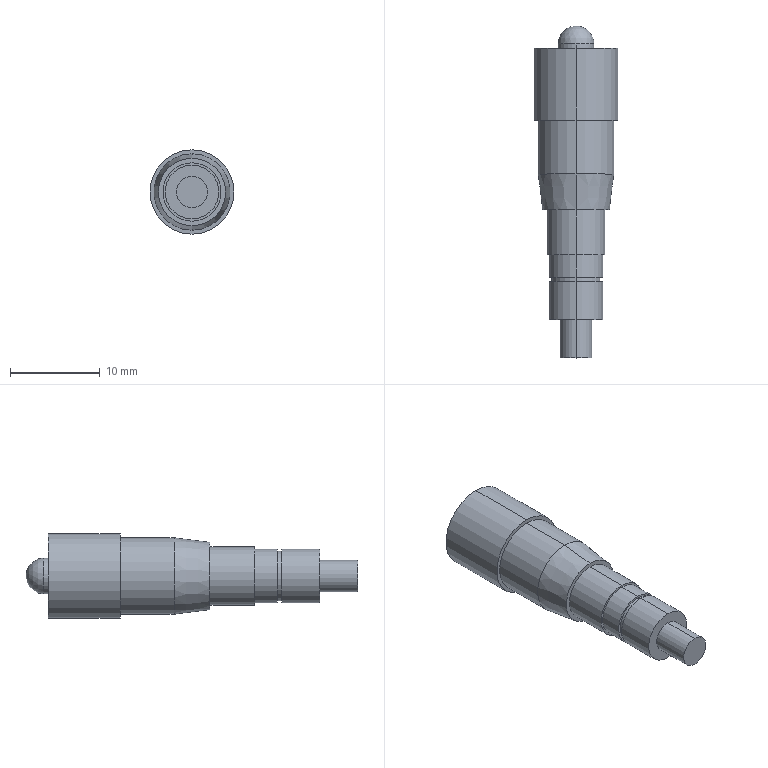Part | SolidWorks | features ICE 7, Chamfer 1, Extrusion 1, Fillet 1 | 1 solid | 27 faces | box 9.4 x 37 x 9.4 mm | volume 1530 mm3 | cylinder 16 | plane 8 | cone 2 | sphere 1 | commonest cylinder face diameters 6 x4 3.5 x2 4 x2 5.5 x2 6.5 x2 8.5 x2
STEP:
#1=CARTESIAN_POINT('',(0.,35.,-2.));
#2=VERTEX_POINT('',#1);
#3=CARTESIAN_POINT('',(0.,35.,2.));
#4=VERTEX_POINT('',#3);
#5=CARTESIAN_POINT('',(0.,35.,0.));
#6=DIRECTION('',(0.,-1.,0.));
#7=DIRECTION('',(0.,0.,-1.));
#8=AXIS2_PLACEMENT_3D('',#5,#6,#7);
#9=CIRCLE('',#8,2.);
#10=EDGE_CURVE('',#2,#4,#9,.T.);
#11=ORIENTED_EDGE('',*,*,#10,.T.);
#12=CARTESIAN_POINT('',(0.,34.5,2.));
#13=VERTEX_POINT('',#12);
#14=CARTESIAN_POINT('',(0.,37.,2.));
#15=DIRECTION('',(0.,-1.,0.));
#16=VECTOR('',#15,1000.);
#17=LINE('',#14,#16);
#18=EDGE_CURVE('',#4,#13,#17,.T.);
#19=ORIENTED_EDGE('',*,*,#18,.T.);
#20=CARTESIAN_POINT('',(0.,34.5,-2.));
#21=VERTEX_POINT('',#20);
#22=CARTESIAN_POINT('',(0.,34.5,0.));
#23=DIRECTION('',(0.,1.,0.));
#24=DIRECTION('',(0.,0.,1.));
#25=AXIS2_PLACEMENT_3D('',#22,#23,#24);
#26=CIRCLE('',#25,2.);
#27=EDGE_CURVE('',#13,#21,#26,.T.);
#28=ORIENTED_EDGE('',*,*,#27,.T.);
#29=CARTESIAN_POINT('',(0.,37.,-2.));
#30=DIRECTION('',(0.,-1.,0.));
#31=VECTOR('',#30,1000.);
#32=LINE('',#29,#31);
#33=EDGE_CURVE('',#2,#21,#32,.T.);
#34=ORIENTED_EDGE('',*,*,#33,.F.);
#35=EDGE_LOOP('',(#11,#19,#28,#34));
#36=FACE_OUTER_BOUND('',#35,.T.);
#37=CARTESIAN_POINT('',(0.,37.,0.));
#38=DIRECTION('',(0.,-1.,0.));
#39=DIRECTION('',(0.,0.,-1.));
#40=AXIS2_PLACEMENT_3D('',#37,#38,#39);
#41=CYLINDRICAL_SURFACE('',#40,2.);
#42=ADVANCED_FACE('',(#36),#41,.T.);
#43=CARTESIAN_POINT('',(0.,34.5,4.7));
#44=VERTEX_POINT('',#43);
#45=CARTESIAN_POINT('',(0.,34.5,-4.7));
#46=VERTEX_POINT('',#45);
#47=CARTESIAN_POINT('',(0.,34.5,0.));
#48=DIRECTION('',(0.,1.,0.));
#49=DIRECTION('',(0.,0.,1.));
#50=AXIS2_PLACEMENT_3D('',#47,#48,#49);
#51=CIRCLE('',#50,4.7);
#52=EDGE_CURVE('',#44,#46,#51,.T.);
#53=ORIENTED_EDGE('',*,*,#52,.F.);
#54=CARTESIAN_POINT('',(0.,26.5,4.7));
#55=VERTEX_POINT('',#54);
#56=CARTESIAN_POINT('',(0.,34.5,4.7));
#57=DIRECTION('',(0.,-1.,0.));
#58=VECTOR('',#57,1000.);
#59=LINE('',#56,#58);
#60=EDGE_CURVE('',#44,#55,#59,.T.);
#61=ORIENTED_EDGE('',*,*,#60,.T.);
#62=CARTESIAN_POINT('',(0.,26.5,-4.7));
#63=VERTEX_POINT('',#62);
#64=CARTESIAN_POINT('',(0.,26.5,0.));
#65=DIRECTION('',(0.,1.,0.));
#66=DIRECTION('',(0.,0.,1.));
#67=AXIS2_PLACEMENT_3D('',#64,#65,#66);
#68=CIRCLE('',#67,4.7);
#69=EDGE_CURVE('',#55,#63,#68,.T.);
#70=ORIENTED_EDGE('',*,*,#69,.T.);
#71=CARTESIAN_POINT('',(0.,34.5,-4.7));
#72=DIRECTION('',(0.,-1.,0.));
#73=VECTOR('',#72,1000.);
#74=LINE('',#71,#73);
#75=EDGE_CURVE('',#46,#63,#74,.T.);
#76=ORIENTED_EDGE('',*,*,#75,.F.);
#77=EDGE_LOOP('',(#53,#61,#70,#76));
#78=FACE_OUTER_BOUND('',#77,.T.);
#79=CARTESIAN_POINT('',(0.,34.5,0.));
#80=DIRECTION('',(0.,-1.,0.));
#81=DIRECTION('',(0.,0.,-1.));
#82=AXIS2_PLACEMENT_3D('',#79,#80,#81);
#83=CYLINDRICAL_SURFACE('',#82,4.7);
#84=ADVANCED_FACE('',(#78),#83,.T.);
#85=CARTESIAN_POINT('',(0.,16.5,-3.75));
#86=VERTEX_POINT('',#85);
#87=CARTESIAN_POINT('',(0.,16.5,3.75));
#88=VERTEX_POINT('',#87);
#89=CARTESIAN_POINT('',(0.,16.5,0.));
#90=DIRECTION('',(0.,-1.,0.));
#91=DIRECTION('',(0.,0.,1.));
#92=AXIS2_PLACEMENT_3D('',#89,#90,#91);
#93=CIRCLE('',#92,3.75);
#94=EDGE_CURVE('',#86,#88,#93,.T.);
#95=ORIENTED_EDGE('',*,*,#94,.F.);
#96=CARTESIAN_POINT('',(0.,20.5,-4.25));
#97=VERTEX_POINT('',#96);
#98=CARTESIAN_POINT('',(0.,20.5,-4.25));
#99=DIRECTION('',(0.,0.9923,-0.124));
#100=VECTOR('',#99,1000.);
#101=LINE('',#98,#100);
#102=EDGE_CURVE('',#86,#97,#101,.T.);
#103=ORIENTED_EDGE('',*,*,#102,.T.);
#104=CARTESIAN_POINT('',(0.,20.5,4.25));
#105=VERTEX_POINT('',#104);
#106=CARTESIAN_POINT('',(0.,20.5,0.));
#107=DIRECTION('',(0.,1.,0.));
#108=DIRECTION('',(0.,0.,1.));
#109=AXIS2_PLACEMENT_3D('',#106,#107,#108);
#110=CIRCLE('',#109,4.25);
#111=EDGE_CURVE('',#105,#97,#110,.T.);
#112=ORIENTED_EDGE('',*,*,#111,.F.);
#113=CARTESIAN_POINT('',(0.,20.5,4.25));
#114=DIRECTION('',(0.,0.9923,0.124));
#115=VECTOR('',#114,1000.);
#116=LINE('',#113,#115);
#117=EDGE_CURVE('',#88,#105,#116,.T.);
#118=ORIENTED_EDGE('',*,*,#117,.F.);
#119=EDGE_LOOP('',(#95,#103,#112,#118));
#120=FACE_OUTER_BOUND('',#119,.T.);
#121=CARTESIAN_POINT('',(0.,20.5,0.));
#122=DIRECTION('',(0.,1.,0.));
#123=DIRECTION('',(0.,0.,1.));
#124=AXIS2_PLACEMENT_3D('',#121,#122,#123);
#125=CONICAL_SURFACE('',#124,4.25,0.1244);
#126=ADVANCED_FACE('',(#120),#125,.T.);
#127=CARTESIAN_POINT('',(0.,26.5,4.25));
#128=VERTEX_POINT('',#127);
#129=CARTESIAN_POINT('',(0.,26.5,-4.25));
#130=VERTEX_POINT('',#129);
#131=CARTESIAN_POINT('',(0.,26.5,0.));
#132=DIRECTION('',(0.,1.,0.));
#133=DIRECTION('',(0.,0.,1.));
#134=AXIS2_PLACEMENT_3D('',#131,#132,#133);
#135=CIRCLE('',#134,4.25);
#136=EDGE_CURVE('',#128,#130,#135,.T.);
#137=ORIENTED_EDGE('',*,*,#136,.F.);
#138=CARTESIAN_POINT('',(0.,26.5,4.25));
#139=DIRECTION('',(0.,-1.,0.));
#140=VECTOR('',#139,1000.);
#141=LINE('',#138,#140);
#142=EDGE_CURVE('',#128,#105,#141,.T.);
#143=ORIENTED_EDGE('',*,*,#142,.T.);
#144=ORIENTED_EDGE('',*,*,#111,.T.);
#145=CARTESIAN_POINT('',(0.,26.5,-4.25));
#146=DIRECTION('',(0.,-1.,0.));
#147=VECTOR('',#146,1000.);
#148=LINE('',#145,#147);
#149=EDGE_CURVE('',#130,#97,#148,.T.);
#150=ORIENTED_EDGE('',*,*,#149,.F.);
#151=EDGE_LOOP('',(#137,#143,#144,#150));
#152=FACE_OUTER_BOUND('',#151,.T.);
#153=CARTESIAN_POINT('',(0.,26.5,0.));
#154=DIRECTION('',(0.,-1.,0.));
#155=DIRECTION('',(0.,0.,-1.));
#156=AXIS2_PLACEMENT_3D('',#153,#154,#155);
#157=CYLINDRICAL_SURFACE('',#156,4.25);
#158=ADVANCED_FACE('',(#152),#157,.T.);
#159=CARTESIAN_POINT('',(0.,16.5,3.25));
#160=VERTEX_POINT('',#159);
#161=CARTESIAN_POINT('',(0.,16.5,-3.25));
#162=VERTEX_POINT('',#161);
#163=CARTESIAN_POINT('',(0.,16.5,0.));
#164=DIRECTION('',(0.,1.,0.));
#165=DIRECTION('',(0.,0.,1.));
#166=AXIS2_PLACEMENT_3D('',#163,#164,#165);
#167=CIRCLE('',#166,3.25);
#168=EDGE_CURVE('',#160,#162,#167,.T.);
#169=ORIENTED_EDGE('',*,*,#168,.F.);
#170=CARTESIAN_POINT('',(0.,11.5,3.25));
#171=VERTEX_POINT('',#170);
#172=CARTESIAN_POINT('',(0.,16.5,3.25));
#173=DIRECTION('',(0.,-1.,0.));
#174=VECTOR('',#173,1000.);
#175=LINE('',#172,#174);
#176=EDGE_CURVE('',#160,#171,#175,.T.);
#177=ORIENTED_EDGE('',*,*,#176,.T.);
#178=CARTESIAN_POINT('',(0.,11.5,-3.25));
#179=VERTEX_POINT('',#178);
#180=CARTESIAN_POINT('',(0.,11.5,0.));
#181=DIRECTION('',(0.,1.,0.));
#182=DIRECTION('',(0.,0.,1.));
#183=AXIS2_PLACEMENT_3D('',#180,#181,#182);
#184=CIRCLE('',#183,3.25);
#185=EDGE_CURVE('',#171,#179,#184,.T.);
#186=ORIENTED_EDGE('',*,*,#185,.T.);
#187=CARTESIAN_POINT('',(0.,16.5,-3.25));
#188=DIRECTION('',(0.,-1.,0.));
#189=VECTOR('',#188,1000.);
#190=LINE('',#187,#189);
#191=EDGE_CURVE('',#162,#179,#190,.T.);
#192=ORIENTED_EDGE('',*,*,#191,.F.);
#193=EDGE_LOOP('',(#169,#177,#186,#192));
#194=FACE_OUTER_BOUND('',#193,.T.);
#195=CARTESIAN_POINT('',(0.,16.5,0.));
#196=DIRECTION('',(0.,-1.,0.));
#197=DIRECTION('',(0.,0.,-1.));
#198=AXIS2_PLACEMENT_3D('',#195,#196,#197);
#199=CYLINDRICAL_SURFACE('',#198,3.25);
#200=ADVANCED_FACE('',(#194),#199,.T.);
#201=CARTESIAN_POINT('',(0.,11.5,3.));
#202=VERTEX_POINT('',#201);
#203=CARTESIAN_POINT('',(0.,11.5,-3.));
#204=VERTEX_POINT('',#203);
#205=CARTESIAN_POINT('',(0.,11.5,0.));
#206=DIRECTION('',(0.,1.,0.));
#207=DIRECTION('',(0.,0.,1.));
#208=AXIS2_PLACEMENT_3D('',#205,#206,#207);
#209=CIRCLE('',#208,3.);
#210=EDGE_CURVE('',#202,#204,#209,.T.);
#211=ORIENTED_EDGE('',*,*,#210,.F.);
#212=CARTESIAN_POINT('',(0.,9.,3.));
#213=VERTEX_POINT('',#212);
#214=CARTESIAN_POINT('',(0.,11.5,3.));
#215=DIRECTION('',(0.,-1.,0.));
#216=VECTOR('',#215,1000.);
#217=LINE('',#214,#216);
#218=EDGE_CURVE('',#202,#213,#217,.T.);
#219=ORIENTED_EDGE('',*,*,#218,.T.);
#220=CARTESIAN_POINT('',(0.,9.,-3.));
#221=VERTEX_POINT('',#220);
#222=CARTESIAN_POINT('',(0.,9.,0.));
#223=DIRECTION('',(0.,1.,0.));
#224=DIRECTION('',(0.,0.,1.));
#225=AXIS2_PLACEMENT_3D('',#222,#223,#224);
#226=CIRCLE('',#225,3.);
#227=EDGE_CURVE('',#213,#221,#226,.T.);
#228=ORIENTED_EDGE('',*,*,#227,.T.);
#229=CARTESIAN_POINT('',(0.,11.5,-3.));
#230=DIRECTION('',(0.,-1.,0.));
#231=VECTOR('',#230,1000.);
#232=LINE('',#229,#231);
#233=EDGE_CURVE('',#204,#221,#232,.T.);
#234=ORIENTED_EDGE('',*,*,#233,.F.);
#235=EDGE_LOOP('',(#211,#219,#228,#234));
#236=FACE_OUTER_BOUND('',#235,.T.);
#237=CARTESIAN_POINT('',(0.,11.5,0.));
#238=DIRECTION('',(0.,-1.,0.));
#239=DIRECTION('',(0.,0.,-1.));
#240=AXIS2_PLACEMENT_3D('',#237,#238,#239);
#241=CYLINDRICAL_SURFACE('',#240,3.);
#242=ADVANCED_FACE('',(#236),#241,.T.);
#243=CARTESIAN_POINT('',(0.,9.,2.75));
#244=VERTEX_POINT('',#243);
#245=CARTESIAN_POINT('',(0.,9.,-2.75));
#246=VERTEX_POINT('',#245);
#247=CARTESIAN_POINT('',(0.,9.,0.));
#248=DIRECTION('',(0.,1.,0.));
#249=DIRECTION('',(0.,0.,1.));
#250=AXIS2_PLACEMENT_3D('',#247,#248,#249);
#251=CIRCLE('',#250,2.75);
#252=EDGE_CURVE('',#244,#246,#251,.T.);
#253=ORIENTED_EDGE('',*,*,#252,.F.);
#254=CARTESIAN_POINT('',(0.,8.5,2.75));
#255=VERTEX_POINT('',#254);
#256=CARTESIAN_POINT('',(0.,9.,2.75));
#257=DIRECTION('',(0.,-1.,0.));
#258=VECTOR('',#257,1000.);
#259=LINE('',#256,#258);
#260=EDGE_CURVE('',#244,#255,#259,.T.);
#261=ORIENTED_EDGE('',*,*,#260,.T.);
#262=CARTESIAN_POINT('',(0.,8.5,-2.75));
#263=VERTEX_POINT('',#262);
#264=CARTESIAN_POINT('',(0.,8.5,0.));
#265=DIRECTION('',(0.,1.,0.));
#266=DIRECTION('',(0.,0.,1.));
#267=AXIS2_PLACEMENT_3D('',#264,#265,#266);
#268=CIRCLE('',#267,2.75);
#269=EDGE_CURVE('',#255,#263,#268,.T.);
#270=ORIENTED_EDGE('',*,*,#269,.T.);
#271=CARTESIAN_POINT('',(0.,9.,-2.75));
#272=DIRECTION('',(0.,-1.,0.));
#273=VECTOR('',#272,1000.);
#274=LINE('',#271,#273);
#275=EDGE_CURVE('',#246,#263,#274,.T.);
#276=ORIENTED_EDGE('',*,*,#275,.F.);
#277=EDGE_LOOP('',(#253,#261,#270,#276));
#278=FACE_OUTER_BOUND('',#277,.T.);
#279=CARTESIAN_POINT('',(0.,9.,0.));
#280=DIRECTION('',(0.,-1.,0.));
#281=DIRECTION('',(0.,0.,-1.));
#282=AXIS2_PLACEMENT_3D('',#279,#280,#281);
#283=CYLINDRICAL_SURFACE('',#282,2.75);
#284=ADVANCED_FACE('',(#278),#283,.T.);
#285=CARTESIAN_POINT('',(0.,8.5,3.));
#286=VERTEX_POINT('',#285);
#287=CARTESIAN_POINT('',(0.,8.5,-3.));
#288=VERTEX_POINT('',#287);
#289=CARTESIAN_POINT('',(0.,8.5,0.));
#290=DIRECTION('',(0.,1.,0.));
#291=DIRECTION('',(0.,0.,1.));
#292=AXIS2_PLACEMENT_3D('',#289,#290,#291);
#293=CIRCLE('',#292,3.);
#294=EDGE_CURVE('',#286,#288,#293,.T.);
#295=ORIENTED_EDGE('',*,*,#294,.F.);
#296=CARTESIAN_POINT('',(0.,4.25,3.));
#297=VERTEX_POINT('',#296);
#298=CARTESIAN_POINT('',(0.,8.5,3.));
#299=DIRECTION('',(0.,-1.,0.));
#300=VECTOR('',#299,1000.);
#301=LINE('',#298,#300);
#302=EDGE_CURVE('',#286,#297,#301,.T.);
#303=ORIENTED_EDGE('',*,*,#302,.T.);
#304=CARTESIAN_POINT('',(0.,4.25,-3.));
#305=VERTEX_POINT('',#304);
#306=CARTESIAN_POINT('',(0.,4.25,0.));
#307=DIRECTION('',(0.,1.,0.));
#308=DIRECTION('',(0.,0.,1.));
#309=AXIS2_PLACEMENT_3D('',#306,#307,#308);
#310=CIRCLE('',#309,3.);
#311=EDGE_CURVE('',#297,#305,#310,.T.);
#312=ORIENTED_EDGE('',*,*,#311,.T.);
#313=CARTESIAN_POINT('',(0.,8.5,-3.));
#314=DIRECTION('',(0.,-1.,0.));
#315=VECTOR('',#314,1000.);
#316=LINE('',#313,#315);
#317=EDGE_CURVE('',#288,#305,#316,.T.);
#318=ORIENTED_EDGE('',*,*,#317,.F.);
#319=EDGE_LOOP('',(#295,#303,#312,#318));
#320=FACE_OUTER_BOUND('',#319,.T.);
#321=CARTESIAN_POINT('',(0.,8.5,0.));
#322=DIRECTION('',(0.,-1.,0.));
#323=DIRECTION('',(0.,0.,-1.));
#324=AXIS2_PLACEMENT_3D('',#321,#322,#323);
#325=CYLINDRICAL_SURFACE('',#324,3.);
#326=ADVANCED_FACE('',(#320),#325,.T.);
#327=CARTESIAN_POINT('',(0.,4.25,1.75));
#328=VERTEX_POINT('',#327);
#329=CARTESIAN_POINT('',(0.,4.25,-1.75));
#330=VERTEX_POINT('',#329);
#331=CARTESIAN_POINT('',(0.,4.25,0.));
#332=DIRECTION('',(0.,1.,0.));
#333=DIRECTION('',(0.,0.,1.));
#334=AXIS2_PLACEMENT_3D('',#331,#332,#333);
#335=CIRCLE('',#334,1.75);
#336=EDGE_CURVE('',#328,#330,#335,.T.);
#337=ORIENTED_EDGE('',*,*,#336,.F.);
#338=CARTESIAN_POINT('',(0.,0.,1.75));
#339=VERTEX_POINT('',#338);
#340=CARTESIAN_POINT('',(0.,4.25,1.75));
#341=DIRECTION('',(0.,-1.,0.));
#342=VECTOR('',#341,1000.);
#343=LINE('',#340,#342);
#344=EDGE_CURVE('',#328,#339,#343,.T.);
#345=ORIENTED_EDGE('',*,*,#344,.T.);
#346=CARTESIAN_POINT('',(0.,0.,-1.75));
#347=VERTEX_POINT('',#346);
#348=CARTESIAN_POINT('',(0.,0.,0.));
#349=DIRECTION('',(0.,1.,0.));
#350=DIRECTION('',(0.,0.,1.));
#351=AXIS2_PLACEMENT_3D('',#348,#349,#350);
#352=CIRCLE('',#351,1.75);
#353=EDGE_CURVE('',#339,#347,#352,.T.);
#354=ORIENTED_EDGE('',*,*,#353,.T.);
#355=CARTESIAN_POINT('',(0.,4.25,-1.75));
#356=DIRECTION('',(0.,-1.,0.));
#357=VECTOR('',#356,1000.);
#358=LINE('',#355,#357);
#359=EDGE_CURVE('',#330,#347,#358,.T.);
#360=ORIENTED_EDGE('',*,*,#359,.F.);
#361=EDGE_LOOP('',(#337,#345,#354,#360));
#362=FACE_OUTER_BOUND('',#361,.T.);
#363=CARTESIAN_POINT('',(0.,4.25,0.));
#364=DIRECTION('',(0.,-1.,0.));
#365=DIRECTION('',(0.,0.,-1.));
#366=AXIS2_PLACEMENT_3D('',#363,#364,#365);
#367=CYLINDRICAL_SURFACE('',#366,1.75);
#368=ADVANCED_FACE('',(#362),#367,.T.);
#369=CARTESIAN_POINT('',(0.,34.5,0.));
#370=DIRECTION('',(0.,1.,0.));
#371=DIRECTION('',(0.,0.,1.));
#372=AXIS2_PLACEMENT_3D('',#369,#370,#371);
#373=CIRCLE('',#372,4.7);
#374=EDGE_CURVE('',#46,#44,#373,.T.);
#375=ORIENTED_EDGE('',*,*,#374,.T.);
#376=ORIENTED_EDGE('',*,*,#52,.T.);
#377=EDGE_LOOP('',(#375,#376));
#378=FACE_OUTER_BOUND('',#377,.T.);
#379=CARTESIAN_POINT('',(0.,34.5,0.));
#380=DIRECTION('',(0.,1.,0.));
#381=DIRECTION('',(0.,0.,1.));
#382=AXIS2_PLACEMENT_3D('',#379,#380,#381);
#383=CIRCLE('',#382,2.);
#384=EDGE_CURVE('',#21,#13,#383,.T.);
#385=ORIENTED_EDGE('',*,*,#384,.F.);
#386=ORIENTED_EDGE('',*,*,#27,.F.);
#387=EDGE_LOOP('',(#385,#386));
#388=FACE_BOUND('',#387,.T.);
#389=CARTESIAN_POINT('',(0.,34.5,0.));
#390=DIRECTION('',(0.,1.,0.));
#391=DIRECTION('',(0.,0.,1.));
#392=AXIS2_PLACEMENT_3D('',#389,#390,#391);
#393=PLANE('',#392);
#394=ADVANCED_FACE('',(#378,#388),#393,.T.);
#395=CARTESIAN_POINT('',(0.,8.5,0.));
#396=DIRECTION('',(0.,1.,0.));
#397=DIRECTION('',(0.,0.,1.));
#398=AXIS2_PLACEMENT_3D('',#395,#396,#397);
#399=CIRCLE('',#398,3.);
#400=EDGE_CURVE('',#288,#286,#399,.T.);
#401=ORIENTED_EDGE('',*,*,#400,.T.);
#402=ORIENTED_EDGE('',*,*,#294,.T.);
#403=EDGE_LOOP('',(#401,#402));
#404=FACE_OUTER_BOUND('',#403,.T.);
#405=CARTESIAN_POINT('',(0.,8.5,0.));
#406=DIRECTION('',(0.,1.,0.));
#407=DIRECTION('',(0.,0.,1.));
#408=AXIS2_PLACEMENT_3D('',#405,#406,#407);
#409=CIRCLE('',#408,2.75);
#410=EDGE_CURVE('',#263,#255,#409,.T.);
#411=ORIENTED_EDGE('',*,*,#410,.F.);
#412=ORIENTED_EDGE('',*,*,#269,.F.);
#413=EDGE_LOOP('',(#411,#412));
#414=FACE_BOUND('',#413,.T.);
#415=CARTESIAN_POINT('',(0.,8.5,0.));
#416=DIRECTION('',(0.,1.,0.));
#417=DIRECTION('',(0.,0.,1.));
#418=AXIS2_PLACEMENT_3D('',#415,#416,#417);
#419=PLANE('',#418);
#420=ADVANCED_FACE('',(#404,#414),#419,.T.);
#421=ORIENTED_EDGE('',*,*,#344,.F.);
#422=CARTESIAN_POINT('',(0.,4.25,0.));
#423=DIRECTION('',(0.,1.,0.));
#424=DIRECTION('',(0.,0.,1.));
#425=AXIS2_PLACEMENT_3D('',#422,#423,#424);
#426=CIRCLE('',#425,1.75);
#427=EDGE_CURVE('',#330,#328,#426,.T.);
#428=ORIENTED_EDGE('',*,*,#427,.F.);
#429=ORIENTED_EDGE('',*,*,#359,.T.);
#430=CARTESIAN_POINT('',(0.,0.,0.));
#431=DIRECTION('',(0.,1.,0.));
#432=DIRECTION('',(0.,0.,1.));
#433=AXIS2_PLACEMENT_3D('',#430,#431,#432);
#434=CIRCLE('',#433,1.75);
#435=EDGE_CURVE('',#347,#339,#434,.T.);
#436=ORIENTED_EDGE('',*,*,#435,.T.);
#437=EDGE_LOOP('',(#421,#428,#429,#436));
#438=FACE_OUTER_BOUND('',#437,.T.);
#439=CARTESIAN_POINT('',(0.,4.25,0.));
#440=DIRECTION('',(0.,-1.,0.));
#441=DIRECTION('',(0.,0.,-1.));
#442=AXIS2_PLACEMENT_3D('',#439,#440,#441);
#443=CYLINDRICAL_SURFACE('',#442,1.75);
#444=ADVANCED_FACE('',(#438),#443,.T.);
#445=ORIENTED_EDGE('',*,*,#435,.F.);
#446=ORIENTED_EDGE('',*,*,#353,.F.);
#447=EDGE_LOOP('',(#445,#446));
#448=FACE_OUTER_BOUND('',#447,.T.);
#449=CARTESIAN_POINT('',(0.,0.,0.));
#450=DIRECTION('',(0.,1.,0.));
#451=DIRECTION('',(0.,0.,1.));
#452=AXIS2_PLACEMENT_3D('',#449,#450,#451);
#453=PLANE('',#452);
#454=ADVANCED_FACE('',(#448),#453,.F.);
#455=CARTESIAN_POINT('',(0.,4.25,0.));
#456=DIRECTION('',(0.,1.,0.));
#457=DIRECTION('',(0.,0.,1.));
#458=AXIS2_PLACEMENT_3D('',#455,#456,#457);
#459=CIRCLE('',#458,3.);
#460=EDGE_CURVE('',#305,#297,#459,.T.);
#461=ORIENTED_EDGE('',*,*,#460,.F.);
#462=ORIENTED_EDGE('',*,*,#311,.F.);
#463=EDGE_LOOP('',(#461,#462));
#464=FACE_OUTER_BOUND('',#463,.T.);
#465=ORIENTED_EDGE('',*,*,#427,.T.);
#466=ORIENTED_EDGE('',*,*,#336,.T.);
#467=EDGE_LOOP('',(#465,#466));
#468=FACE_BOUND('',#467,.T.);
#469=CARTESIAN_POINT('',(0.,4.25,0.));
#470=DIRECTION('',(0.,1.,0.));
#471=DIRECTION('',(0.,0.,1.));
#472=AXIS2_PLACEMENT_3D('',#469,#470,#471);
#473=PLANE('',#472);
#474=ADVANCED_FACE('',(#464,#468),#473,.F.);
#475=ORIENTED_EDGE('',*,*,#302,.F.);
#476=ORIENTED_EDGE('',*,*,#400,.F.);
#477=ORIENTED_EDGE('',*,*,#317,.T.);
#478=ORIENTED_EDGE('',*,*,#460,.T.);
#479=EDGE_LOOP('',(#475,#476,#477,#478));
#480=FACE_OUTER_BOUND('',#479,.T.);
#481=CARTESIAN_POINT('',(0.,8.5,0.));
#482=DIRECTION('',(0.,-1.,0.));
#483=DIRECTION('',(0.,0.,-1.));
#484=AXIS2_PLACEMENT_3D('',#481,#482,#483);
#485=CYLINDRICAL_SURFACE('',#484,3.);
#486=ADVANCED_FACE('',(#480),#485,.T.);
#487=ORIENTED_EDGE('',*,*,#260,.F.);
#488=CARTESIAN_POINT('',(0.,9.,0.));
#489=DIRECTION('',(0.,1.,0.));
#490=DIRECTION('',(0.,0.,1.));
#491=AXIS2_PLACEMENT_3D('',#488,#489,#490);
#492=CIRCLE('',#491,2.75);
#493=EDGE_CURVE('',#246,#244,#492,.T.);
#494=ORIENTED_EDGE('',*,*,#493,.F.);
#495=ORIENTED_EDGE('',*,*,#275,.T.);
#496=ORIENTED_EDGE('',*,*,#410,.T.);
#497=EDGE_LOOP('',(#487,#494,#495,#496));
#498=FACE_OUTER_BOUND('',#497,.T.);
#499=CARTESIAN_POINT('',(0.,9.,0.));
#500=DIRECTION('',(0.,-1.,0.));
#501=DIRECTION('',(0.,0.,-1.));
#502=AXIS2_PLACEMENT_3D('',#499,#500,#501);
#503=CYLINDRICAL_SURFACE('',#502,2.75);
#504=ADVANCED_FACE('',(#498),#503,.T.);
#505=CARTESIAN_POINT('',(0.,9.,0.));
#506=DIRECTION('',(0.,1.,0.));
#507=DIRECTION('',(0.,0.,1.));
#508=AXIS2_PLACEMENT_3D('',#505,#506,#507);
#509=CIRCLE('',#508,3.);
#510=EDGE_CURVE('',#221,#213,#509,.T.);
#511=ORIENTED_EDGE('',*,*,#510,.F.);
#512=ORIENTED_EDGE('',*,*,#227,.F.);
#513=EDGE_LOOP('',(#511,#512));
#514=FACE_OUTER_BOUND('',#513,.T.);
#515=ORIENTED_EDGE('',*,*,#493,.T.);
#516=ORIENTED_EDGE('',*,*,#252,.T.);
#517=EDGE_LOOP('',(#515,#516));
#518=FACE_BOUND('',#517,.T.);
#519=CARTESIAN_POINT('',(0.,9.,0.));
#520=DIRECTION('',(0.,1.,0.));
#521=DIRECTION('',(0.,0.,1.));
#522=AXIS2_PLACEMENT_3D('',#519,#520,#521);
#523=PLANE('',#522);
#524=ADVANCED_FACE('',(#514,#518),#523,.F.);
#525=ORIENTED_EDGE('',*,*,#218,.F.);
#526=CARTESIAN_POINT('',(0.,11.5,0.));
#527=DIRECTION('',(0.,1.,0.));
#528=DIRECTION('',(0.,0.,1.));
#529=AXIS2_PLACEMENT_3D('',#526,#527,#528);
#530=CIRCLE('',#529,3.);
#531=EDGE_CURVE('',#204,#202,#530,.T.);
#532=ORIENTED_EDGE('',*,*,#531,.F.);
#533=ORIENTED_EDGE('',*,*,#233,.T.);
#534=ORIENTED_EDGE('',*,*,#510,.T.);
#535=EDGE_LOOP('',(#525,#532,#533,#534));
#536=FACE_OUTER_BOUND('',#535,.T.);
#537=CARTESIAN_POINT('',(0.,11.5,0.));
#538=DIRECTION('',(0.,-1.,0.));
#539=DIRECTION('',(0.,0.,-1.));
#540=AXIS2_PLACEMENT_3D('',#537,#538,#539);
#541=CYLINDRICAL_SURFACE('',#540,3.);
#542=ADVANCED_FACE('',(#536),#541,.T.);
#543=CARTESIAN_POINT('',(0.,11.5,0.));
#544=DIRECTION('',(0.,1.,0.));
#545=DIRECTION('',(0.,0.,1.));
#546=AXIS2_PLACEMENT_3D('',#543,#544,#545);
#547=CIRCLE('',#546,3.25);
#548=EDGE_CURVE('',#179,#171,#547,.T.);
#549=ORIENTED_EDGE('',*,*,#548,.F.);
#550=ORIENTED_EDGE('',*,*,#185,.F.);
#551=EDGE_LOOP('',(#549,#550));
#552=FACE_OUTER_BOUND('',#551,.T.);
#553=ORIENTED_EDGE('',*,*,#531,.T.);
#554=ORIENTED_EDGE('',*,*,#210,.T.);
#555=EDGE_LOOP('',(#553,#554));
#556=FACE_BOUND('',#555,.T.);
#557=CARTESIAN_POINT('',(0.,11.5,0.));
#558=DIRECTION('',(0.,1.,0.));
#559=DIRECTION('',(0.,0.,1.));
#560=AXIS2_PLACEMENT_3D('',#557,#558,#559);
#561=PLANE('',#560);
#562=ADVANCED_FACE('',(#552,#556),#561,.F.);
#563=ORIENTED_EDGE('',*,*,#176,.F.);
#564=CARTESIAN_POINT('',(0.,16.5,0.));
#565=DIRECTION('',(0.,1.,0.));
#566=DIRECTION('',(0.,0.,1.));
#567=AXIS2_PLACEMENT_3D('',#564,#565,#566);
#568=CIRCLE('',#567,3.25);
#569=EDGE_CURVE('',#162,#160,#568,.T.);
#570=ORIENTED_EDGE('',*,*,#569,.F.);
#571=ORIENTED_EDGE('',*,*,#191,.T.);
#572=ORIENTED_EDGE('',*,*,#548,.T.);
#573=EDGE_LOOP('',(#563,#570,#571,#572));
#574=FACE_OUTER_BOUND('',#573,.T.);
#575=CARTESIAN_POINT('',(0.,16.5,0.));
#576=DIRECTION('',(0.,-1.,0.));
#577=DIRECTION('',(0.,0.,-1.));
#578=AXIS2_PLACEMENT_3D('',#575,#576,#577);
#579=CYLINDRICAL_SURFACE('',#578,3.25);
#580=ADVANCED_FACE('',(#574),#579,.T.);
#581=CARTESIAN_POINT('',(0.,16.5,0.));
#582=DIRECTION('',(0.,-1.,0.));
#583=DIRECTION('',(0.,0.,1.));
#584=AXIS2_PLACEMENT_3D('',#581,#582,#583);
#585=CIRCLE('',#584,3.75);
#586=EDGE_CURVE('',#88,#86,#585,.T.);
#587=ORIENTED_EDGE('',*,*,#586,.T.);
#588=ORIENTED_EDGE('',*,*,#94,.T.);
#589=EDGE_LOOP('',(#587,#588));
#590=FACE_OUTER_BOUND('',#589,.T.);
#591=ORIENTED_EDGE('',*,*,#569,.T.);
#592=ORIENTED_EDGE('',*,*,#168,.T.);
#593=EDGE_LOOP('',(#591,#592));
#594=FACE_BOUND('',#593,.T.);
#595=CARTESIAN_POINT('',(0.,16.5,0.));
#596=DIRECTION('',(0.,1.,0.));
#597=DIRECTION('',(0.,0.,1.));
#598=AXIS2_PLACEMENT_3D('',#595,#596,#597);
#599=PLANE('',#598);
#600=ADVANCED_FACE('',(#590,#594),#599,.F.);
#601=ORIENTED_EDGE('',*,*,#142,.F.);
#602=CARTESIAN_POINT('',(0.,26.5,0.));
#603=DIRECTION('',(0.,1.,0.));
#604=DIRECTION('',(0.,0.,1.));
#605=AXIS2_PLACEMENT_3D('',#602,#603,#604);
#606=CIRCLE('',#605,4.25);
#607=EDGE_CURVE('',#130,#128,#606,.T.);
#608=ORIENTED_EDGE('',*,*,#607,.F.);
#609=ORIENTED_EDGE('',*,*,#149,.T.);
#610=CARTESIAN_POINT('',(0.,20.5,0.));
#611=DIRECTION('',(0.,1.,0.));
#612=DIRECTION('',(0.,0.,1.));
#613=AXIS2_PLACEMENT_3D('',#610,#611,#612);
#614=CIRCLE('',#613,4.25);
#615=EDGE_CURVE('',#97,#105,#614,.T.);
#616=ORIENTED_EDGE('',*,*,#615,.T.);
#617=EDGE_LOOP('',(#601,#608,#609,#616));
#618=FACE_OUTER_BOUND('',#617,.T.);
#619=CARTESIAN_POINT('',(0.,26.5,0.));
#620=DIRECTION('',(0.,-1.,0.));
#621=DIRECTION('',(0.,0.,-1.));
#622=AXIS2_PLACEMENT_3D('',#619,#620,#621);
#623=CYLINDRICAL_SURFACE('',#622,4.25);
#624=ADVANCED_FACE('',(#618),#623,.T.);
#625=ORIENTED_EDGE('',*,*,#102,.F.);
#626=ORIENTED_EDGE('',*,*,#586,.F.);
#627=ORIENTED_EDGE('',*,*,#117,.T.);
#628=ORIENTED_EDGE('',*,*,#615,.F.);
#629=EDGE_LOOP('',(#625,#626,#627,#628));
#630=FACE_OUTER_BOUND('',#629,.T.);
#631=CARTESIAN_POINT('',(0.,20.5,0.));
#632=DIRECTION('',(0.,1.,0.));
#633=DIRECTION('',(0.,0.,1.));
#634=AXIS2_PLACEMENT_3D('',#631,#632,#633);
#635=CONICAL_SURFACE('',#634,4.25,0.1244);
#636=ADVANCED_FACE('',(#630),#635,.T.);
#637=CARTESIAN_POINT('',(0.,26.5,0.));
#638=DIRECTION('',(0.,1.,0.));
#639=DIRECTION('',(0.,0.,1.));
#640=AXIS2_PLACEMENT_3D('',#637,#638,#639);
#641=CIRCLE('',#640,4.7);
#642=EDGE_CURVE('',#63,#55,#641,.T.);
#643=ORIENTED_EDGE('',*,*,#642,.F.);
#644=ORIENTED_EDGE('',*,*,#69,.F.);
#645=EDGE_LOOP('',(#643,#644));
#646=FACE_OUTER_BOUND('',#645,.T.);
#647=ORIENTED_EDGE('',*,*,#607,.T.);
#648=ORIENTED_EDGE('',*,*,#136,.T.);
#649=EDGE_LOOP('',(#647,#648));
#650=FACE_BOUND('',#649,.T.);
#651=CARTESIAN_POINT('',(0.,26.5,0.));
#652=DIRECTION('',(0.,1.,0.));
#653=DIRECTION('',(0.,0.,1.));
#654=AXIS2_PLACEMENT_3D('',#651,#652,#653);
#655=PLANE('',#654);
#656=ADVANCED_FACE('',(#646,#650),#655,.F.);
#657=ORIENTED_EDGE('',*,*,#60,.F.);
#658=ORIENTED_EDGE('',*,*,#374,.F.);
#659=ORIENTED_EDGE('',*,*,#75,.T.);
#660=ORIENTED_EDGE('',*,*,#642,.T.);
#661=EDGE_LOOP('',(#657,#658,#659,#660));
#662=FACE_OUTER_BOUND('',#661,.T.);
#663=CARTESIAN_POINT('',(0.,34.5,0.));
#664=DIRECTION('',(0.,-1.,0.));
#665=DIRECTION('',(0.,0.,-1.));
#666=AXIS2_PLACEMENT_3D('',#663,#664,#665);
#667=CYLINDRICAL_SURFACE('',#666,4.7);
#668=ADVANCED_FACE('',(#662),#667,.T.);
#669=ORIENTED_EDGE('',*,*,#18,.F.);
#670=CARTESIAN_POINT('',(0.,35.,0.));
#671=DIRECTION('',(0.,-1.,0.));
#672=DIRECTION('',(0.,0.,-1.));
#673=AXIS2_PLACEMENT_3D('',#670,#671,#672);
#674=CIRCLE('',#673,2.);
#675=EDGE_CURVE('',#4,#2,#674,.T.);
#676=ORIENTED_EDGE('',*,*,#675,.T.);
#677=ORIENTED_EDGE('',*,*,#33,.T.);
#678=ORIENTED_EDGE('',*,*,#384,.T.);
#679=EDGE_LOOP('',(#669,#676,#677,#678));
#680=FACE_OUTER_BOUND('',#679,.T.);
#681=CARTESIAN_POINT('',(0.,37.,0.));
#682=DIRECTION('',(0.,-1.,0.));
#683=DIRECTION('',(0.,0.,-1.));
#684=AXIS2_PLACEMENT_3D('',#681,#682,#683);
#685=CYLINDRICAL_SURFACE('',#684,2.);
#686=ADVANCED_FACE('',(#680),#685,.T.);
#687=ORIENTED_EDGE('',*,*,#10,.F.);
#688=ORIENTED_EDGE('',*,*,#675,.F.);
#689=EDGE_LOOP('',(#687,#688));
#690=FACE_OUTER_BOUND('',#689,.T.);
#691=CARTESIAN_POINT('',(0.,35.,0.));
#692=DIRECTION('',(0.,1.,0.));
#693=DIRECTION('',(1.,0.,0.));
#694=AXIS2_PLACEMENT_3D('',#691,#692,#693);
#695=SPHERICAL_SURFACE('',#694,2.);
#696=ADVANCED_FACE('',(#690),#695,.T.);
#697=CLOSED_SHELL('',(#42,#84,#126,#158,#200,#242,#284,#326,#368,#394,#420,#444,#454,#474,#486,#504,#524,#542,#562,#580,#600,#624,#636,#656,#668,#686,#696));
#698=MANIFOLD_SOLID_BREP('',#697);
#699=CARTESIAN_POINT('',(0.,0.,0.));
#700=DIRECTION('',(0.,0.,1.));
#701=DIRECTION('',(1.,0.,0.));
#702=AXIS2_PLACEMENT_3D('',#699,#700,#701);
#703=(LENGTH_UNIT()NAMED_UNIT(*)SI_UNIT(.MILLI.,.METRE.));
#704=UNCERTAINTY_MEASURE_WITH_UNIT(LENGTH_MEASURE(0.00001),#703,'','');
#705=(NAMED_UNIT(*)PLANE_ANGLE_UNIT()SI_UNIT($,.RADIAN.));
#706=(NAMED_UNIT(*)SI_UNIT($,.STERADIAN.)SOLID_ANGLE_UNIT());
#707=(GEOMETRIC_REPRESENTATION_CONTEXT(3)GLOBAL_UNCERTAINTY_ASSIGNED_CONTEXT((#704))GLOBAL_UNIT_ASSIGNED_CONTEXT((#703,#705,#706))REPRESENTATION_CONTEXT('',''));
#708=ADVANCED_BREP_SHAPE_REPRESENTATION('',(#698,#702),#707);